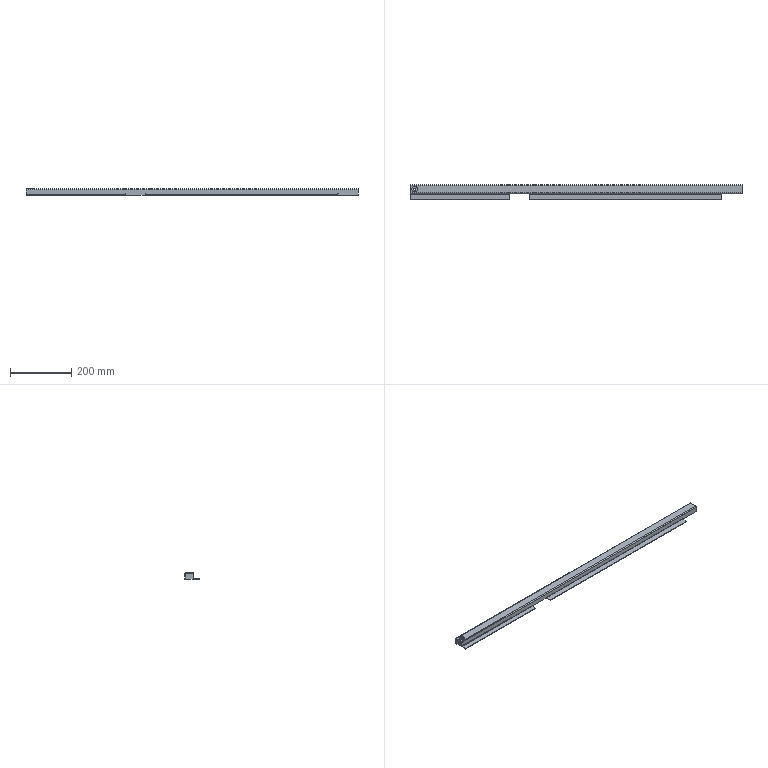Part | SolidWorks | features BaseBody 3 | 3 solids | 81 faces | box 1088 x 48 x 20 mm | volume 174806 mm3 | plane 63 | cylinder 18 | commonest cylinder face diameters 2 x8 6 x6 6.5 x2 18 x2